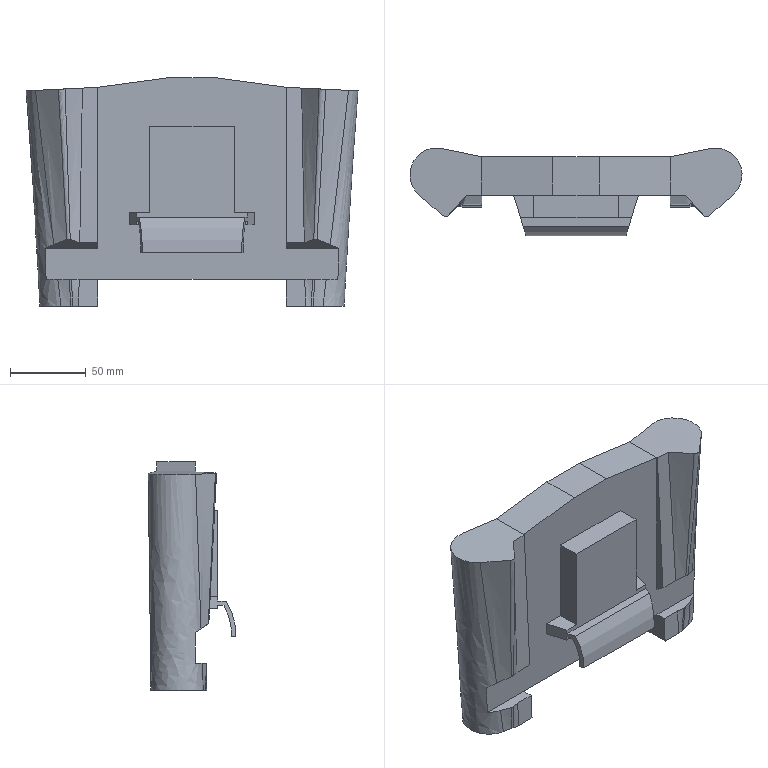Part | NX | features BREP 1 | 1 solid | 62 faces | box 219.713 x 57.963 x 151.13 mm | volume 849978 mm3 | plane 42 | spline 14 | cylinder 6 | commonest cylinder face diameters 14.873 x4 81.86 x1 87.448 x1